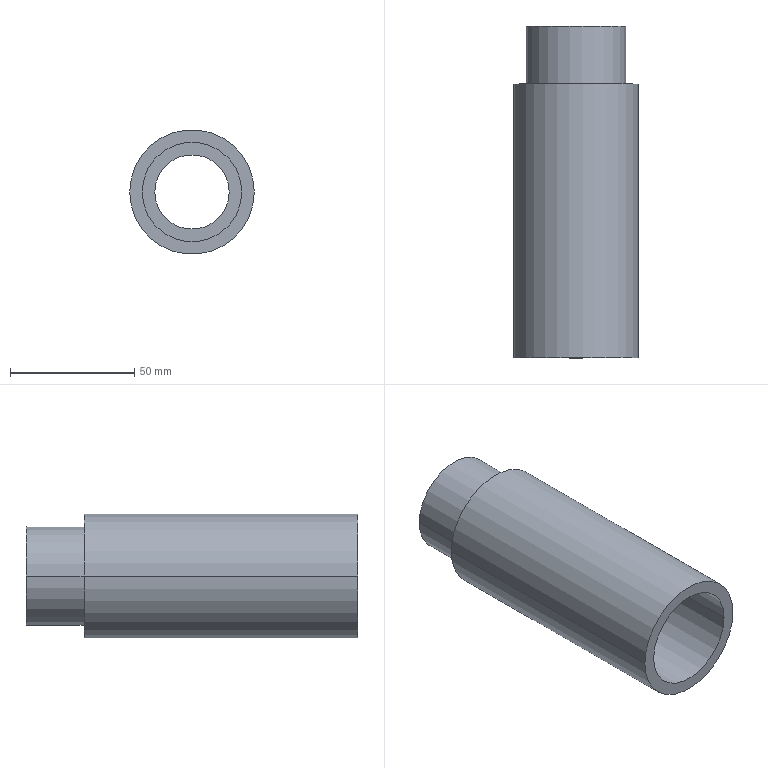Part | SolidWorks | features Revolution 1 | 1 solid | 12 faces | box 50 x 133.28 x 50 mm | volume 92984 mm3 | cylinder 8 | plane 4 | commonest cylinder face diameters 29.9 x2 39.9 x2 40 x2 50 x2
STEP:
#1=CARTESIAN_POINT('',(91.067,-25.489,0.));
#2=VERTEX_POINT('',#1);
#3=CARTESIAN_POINT('',(51.067,-25.489,0.));
#4=VERTEX_POINT('',#3);
#5=CARTESIAN_POINT('',(71.067,-25.489,0.));
#6=DIRECTION('',(0.,1.,0.));
#7=DIRECTION('',(-1.,0.,0.));
#8=AXIS2_PLACEMENT_3D('',#5,#6,#7);
#9=CIRCLE('',#8,20.);
#10=EDGE_CURVE('',#2,#4,#9,.T.);
#11=ORIENTED_EDGE('',*,*,#10,.F.);
#12=CARTESIAN_POINT('',(91.067,80.061,0.));
#13=VERTEX_POINT('',#12);
#14=CARTESIAN_POINT('',(91.067,101.178,0.));
#15=DIRECTION('',(0.,1.,0.));
#16=VECTOR('',#15,1000.);
#17=LINE('',#14,#16);
#18=EDGE_CURVE('',#2,#13,#17,.T.);
#19=ORIENTED_EDGE('',*,*,#18,.T.);
#20=CARTESIAN_POINT('',(51.067,80.061,0.));
#21=VERTEX_POINT('',#20);
#22=CARTESIAN_POINT('',(71.067,80.061,0.));
#23=DIRECTION('',(0.,1.,0.));
#24=DIRECTION('',(-1.,0.,0.));
#25=AXIS2_PLACEMENT_3D('',#22,#23,#24);
#26=CIRCLE('',#25,20.);
#27=EDGE_CURVE('',#13,#21,#26,.T.);
#28=ORIENTED_EDGE('',*,*,#27,.T.);
#29=CARTESIAN_POINT('',(51.067,101.178,0.));
#30=DIRECTION('',(0.,1.,0.));
#31=VECTOR('',#30,1000.);
#32=LINE('',#29,#31);
#33=EDGE_CURVE('',#4,#21,#32,.T.);
#34=ORIENTED_EDGE('',*,*,#33,.F.);
#35=EDGE_LOOP('',(#11,#19,#28,#34));
#36=FACE_OUTER_BOUND('',#35,.T.);
#37=CARTESIAN_POINT('',(71.067,101.178,0.));
#38=DIRECTION('',(0.,1.,0.));
#39=DIRECTION('',(-1.,0.,0.));
#40=AXIS2_PLACEMENT_3D('',#37,#38,#39);
#41=CYLINDRICAL_SURFACE('',#40,20.);
#42=ADVANCED_FACE('',(#36),#41,.F.);
#43=CARTESIAN_POINT('',(86.017,80.061,0.));
#44=VERTEX_POINT('',#43);
#45=CARTESIAN_POINT('',(56.117,80.061,0.));
#46=VERTEX_POINT('',#45);
#47=CARTESIAN_POINT('',(71.067,80.061,0.));
#48=DIRECTION('',(0.,1.,0.));
#49=DIRECTION('',(-1.,0.,0.));
#50=AXIS2_PLACEMENT_3D('',#47,#48,#49);
#51=CIRCLE('',#50,14.95);
#52=EDGE_CURVE('',#44,#46,#51,.T.);
#53=ORIENTED_EDGE('',*,*,#52,.F.);
#54=CARTESIAN_POINT('',(86.017,107.791,0.));
#55=VERTEX_POINT('',#54);
#56=CARTESIAN_POINT('',(86.017,101.178,0.));
#57=DIRECTION('',(0.,1.,0.));
#58=VECTOR('',#57,1000.);
#59=LINE('',#56,#58);
#60=EDGE_CURVE('',#44,#55,#59,.T.);
#61=ORIENTED_EDGE('',*,*,#60,.T.);
#62=CARTESIAN_POINT('',(56.117,107.791,0.));
#63=VERTEX_POINT('',#62);
#64=CARTESIAN_POINT('',(71.067,107.791,0.));
#65=DIRECTION('',(0.,1.,0.));
#66=DIRECTION('',(-1.,0.,0.));
#67=AXIS2_PLACEMENT_3D('',#64,#65,#66);
#68=CIRCLE('',#67,14.95);
#69=EDGE_CURVE('',#55,#63,#68,.T.);
#70=ORIENTED_EDGE('',*,*,#69,.T.);
#71=CARTESIAN_POINT('',(56.117,101.178,0.));
#72=DIRECTION('',(0.,1.,0.));
#73=VECTOR('',#72,1000.);
#74=LINE('',#71,#73);
#75=EDGE_CURVE('',#46,#63,#74,.T.);
#76=ORIENTED_EDGE('',*,*,#75,.F.);
#77=EDGE_LOOP('',(#53,#61,#70,#76));
#78=FACE_OUTER_BOUND('',#77,.T.);
#79=CARTESIAN_POINT('',(71.067,101.178,0.));
#80=DIRECTION('',(0.,1.,0.));
#81=DIRECTION('',(-1.,0.,0.));
#82=AXIS2_PLACEMENT_3D('',#79,#80,#81);
#83=CYLINDRICAL_SURFACE('',#82,14.95);
#84=ADVANCED_FACE('',(#78),#83,.F.);
#85=CARTESIAN_POINT('',(51.117,84.511,0.));
#86=VERTEX_POINT('',#85);
#87=CARTESIAN_POINT('',(91.017,84.511,0.));
#88=VERTEX_POINT('',#87);
#89=CARTESIAN_POINT('',(71.067,84.511,0.));
#90=DIRECTION('',(0.,1.,0.));
#91=DIRECTION('',(-1.,0.,0.));
#92=AXIS2_PLACEMENT_3D('',#89,#90,#91);
#93=CIRCLE('',#92,19.95);
#94=EDGE_CURVE('',#86,#88,#93,.T.);
#95=ORIENTED_EDGE('',*,*,#94,.T.);
#96=CARTESIAN_POINT('',(91.017,107.791,0.));
#97=VERTEX_POINT('',#96);
#98=CARTESIAN_POINT('',(91.017,101.178,0.));
#99=DIRECTION('',(0.,1.,0.));
#100=VECTOR('',#99,1000.);
#101=LINE('',#98,#100);
#102=EDGE_CURVE('',#88,#97,#101,.T.);
#103=ORIENTED_EDGE('',*,*,#102,.T.);
#104=CARTESIAN_POINT('',(51.117,107.791,0.));
#105=VERTEX_POINT('',#104);
#106=CARTESIAN_POINT('',(71.067,107.791,0.));
#107=DIRECTION('',(0.,1.,0.));
#108=DIRECTION('',(-1.,0.,0.));
#109=AXIS2_PLACEMENT_3D('',#106,#107,#108);
#110=CIRCLE('',#109,19.95);
#111=EDGE_CURVE('',#105,#97,#110,.T.);
#112=ORIENTED_EDGE('',*,*,#111,.F.);
#113=CARTESIAN_POINT('',(51.117,101.178,0.));
#114=DIRECTION('',(0.,1.,0.));
#115=VECTOR('',#114,1000.);
#116=LINE('',#113,#115);
#117=EDGE_CURVE('',#86,#105,#116,.T.);
#118=ORIENTED_EDGE('',*,*,#117,.F.);
#119=EDGE_LOOP('',(#95,#103,#112,#118));
#120=FACE_OUTER_BOUND('',#119,.T.);
#121=CARTESIAN_POINT('',(71.067,101.178,0.));
#122=DIRECTION('',(0.,1.,0.));
#123=DIRECTION('',(-1.,0.,0.));
#124=AXIS2_PLACEMENT_3D('',#121,#122,#123);
#125=CYLINDRICAL_SURFACE('',#124,19.95);
#126=ADVANCED_FACE('',(#120),#125,.T.);
#127=CARTESIAN_POINT('',(46.067,-25.489,0.));
#128=VERTEX_POINT('',#127);
#129=CARTESIAN_POINT('',(96.067,-25.489,0.));
#130=VERTEX_POINT('',#129);
#131=CARTESIAN_POINT('',(71.067,-25.489,0.));
#132=DIRECTION('',(0.,1.,0.));
#133=DIRECTION('',(-1.,0.,0.));
#134=AXIS2_PLACEMENT_3D('',#131,#132,#133);
#135=CIRCLE('',#134,25.);
#136=EDGE_CURVE('',#128,#130,#135,.T.);
#137=ORIENTED_EDGE('',*,*,#136,.T.);
#138=CARTESIAN_POINT('',(96.067,84.511,0.));
#139=VERTEX_POINT('',#138);
#140=CARTESIAN_POINT('',(96.067,101.178,0.));
#141=DIRECTION('',(0.,1.,0.));
#142=VECTOR('',#141,1000.);
#143=LINE('',#140,#142);
#144=EDGE_CURVE('',#130,#139,#143,.T.);
#145=ORIENTED_EDGE('',*,*,#144,.T.);
#146=CARTESIAN_POINT('',(46.067,84.511,0.));
#147=VERTEX_POINT('',#146);
#148=CARTESIAN_POINT('',(71.067,84.511,0.));
#149=DIRECTION('',(0.,1.,0.));
#150=DIRECTION('',(-1.,0.,0.));
#151=AXIS2_PLACEMENT_3D('',#148,#149,#150);
#152=CIRCLE('',#151,25.);
#153=EDGE_CURVE('',#147,#139,#152,.T.);
#154=ORIENTED_EDGE('',*,*,#153,.F.);
#155=CARTESIAN_POINT('',(46.067,101.178,0.));
#156=DIRECTION('',(0.,1.,0.));
#157=VECTOR('',#156,1000.);
#158=LINE('',#155,#157);
#159=EDGE_CURVE('',#128,#147,#158,.T.);
#160=ORIENTED_EDGE('',*,*,#159,.F.);
#161=EDGE_LOOP('',(#137,#145,#154,#160));
#162=FACE_OUTER_BOUND('',#161,.T.);
#163=CARTESIAN_POINT('',(71.067,101.178,0.));
#164=DIRECTION('',(0.,1.,0.));
#165=DIRECTION('',(-1.,0.,0.));
#166=AXIS2_PLACEMENT_3D('',#163,#164,#165);
#167=CYLINDRICAL_SURFACE('',#166,25.);
#168=ADVANCED_FACE('',(#162),#167,.T.);
#169=CARTESIAN_POINT('',(71.067,-25.489,0.));
#170=DIRECTION('',(0.,1.,0.));
#171=DIRECTION('',(-1.,0.,0.));
#172=AXIS2_PLACEMENT_3D('',#169,#170,#171);
#173=CIRCLE('',#172,20.);
#174=EDGE_CURVE('',#4,#2,#173,.T.);
#175=ORIENTED_EDGE('',*,*,#174,.T.);
#176=ORIENTED_EDGE('',*,*,#10,.T.);
#177=EDGE_LOOP('',(#175,#176));
#178=FACE_BOUND('',#177,.T.);
#179=ORIENTED_EDGE('',*,*,#136,.F.);
#180=CARTESIAN_POINT('',(71.067,-25.489,0.));
#181=DIRECTION('',(0.,1.,0.));
#182=DIRECTION('',(-1.,0.,0.));
#183=AXIS2_PLACEMENT_3D('',#180,#181,#182);
#184=CIRCLE('',#183,25.);
#185=EDGE_CURVE('',#130,#128,#184,.T.);
#186=ORIENTED_EDGE('',*,*,#185,.F.);
#187=EDGE_LOOP('',(#179,#186));
#188=FACE_OUTER_BOUND('',#187,.T.);
#189=CARTESIAN_POINT('',(51.067,-25.489,0.));
#190=DIRECTION('',(0.,-1.,0.));
#191=DIRECTION('',(1.,0.,0.));
#192=AXIS2_PLACEMENT_3D('',#189,#190,#191);
#193=PLANE('',#192);
#194=ADVANCED_FACE('',(#178,#188),#193,.T.);
#195=ORIENTED_EDGE('',*,*,#144,.F.);
#196=ORIENTED_EDGE('',*,*,#185,.T.);
#197=ORIENTED_EDGE('',*,*,#159,.T.);
#198=CARTESIAN_POINT('',(71.067,84.511,0.));
#199=DIRECTION('',(0.,1.,0.));
#200=DIRECTION('',(-1.,0.,0.));
#201=AXIS2_PLACEMENT_3D('',#198,#199,#200);
#202=CIRCLE('',#201,25.);
#203=EDGE_CURVE('',#139,#147,#202,.T.);
#204=ORIENTED_EDGE('',*,*,#203,.F.);
#205=EDGE_LOOP('',(#195,#196,#197,#204));
#206=FACE_OUTER_BOUND('',#205,.T.);
#207=CARTESIAN_POINT('',(71.067,101.178,0.));
#208=DIRECTION('',(0.,1.,0.));
#209=DIRECTION('',(-1.,0.,0.));
#210=AXIS2_PLACEMENT_3D('',#207,#208,#209);
#211=CYLINDRICAL_SURFACE('',#210,25.);
#212=ADVANCED_FACE('',(#206),#211,.T.);
#213=ORIENTED_EDGE('',*,*,#153,.T.);
#214=ORIENTED_EDGE('',*,*,#203,.T.);
#215=EDGE_LOOP('',(#213,#214));
#216=FACE_OUTER_BOUND('',#215,.T.);
#217=ORIENTED_EDGE('',*,*,#94,.F.);
#218=CARTESIAN_POINT('',(71.067,84.511,0.));
#219=DIRECTION('',(0.,1.,0.));
#220=DIRECTION('',(-1.,0.,0.));
#221=AXIS2_PLACEMENT_3D('',#218,#219,#220);
#222=CIRCLE('',#221,19.95);
#223=EDGE_CURVE('',#88,#86,#222,.T.);
#224=ORIENTED_EDGE('',*,*,#223,.F.);
#225=EDGE_LOOP('',(#217,#224));
#226=FACE_BOUND('',#225,.T.);
#227=CARTESIAN_POINT('',(51.117,84.511,0.));
#228=DIRECTION('',(0.,1.,0.));
#229=DIRECTION('',(-1.,0.,0.));
#230=AXIS2_PLACEMENT_3D('',#227,#228,#229);
#231=PLANE('',#230);
#232=ADVANCED_FACE('',(#216,#226),#231,.T.);
#233=ORIENTED_EDGE('',*,*,#102,.F.);
#234=ORIENTED_EDGE('',*,*,#223,.T.);
#235=ORIENTED_EDGE('',*,*,#117,.T.);
#236=CARTESIAN_POINT('',(71.067,107.791,0.));
#237=DIRECTION('',(0.,1.,0.));
#238=DIRECTION('',(-1.,0.,0.));
#239=AXIS2_PLACEMENT_3D('',#236,#237,#238);
#240=CIRCLE('',#239,19.95);
#241=EDGE_CURVE('',#97,#105,#240,.T.);
#242=ORIENTED_EDGE('',*,*,#241,.F.);
#243=EDGE_LOOP('',(#233,#234,#235,#242));
#244=FACE_OUTER_BOUND('',#243,.T.);
#245=CARTESIAN_POINT('',(71.067,101.178,0.));
#246=DIRECTION('',(0.,1.,0.));
#247=DIRECTION('',(-1.,0.,0.));
#248=AXIS2_PLACEMENT_3D('',#245,#246,#247);
#249=CYLINDRICAL_SURFACE('',#248,19.95);
#250=ADVANCED_FACE('',(#244),#249,.T.);
#251=ORIENTED_EDGE('',*,*,#111,.T.);
#252=ORIENTED_EDGE('',*,*,#241,.T.);
#253=EDGE_LOOP('',(#251,#252));
#254=FACE_OUTER_BOUND('',#253,.T.);
#255=CARTESIAN_POINT('',(71.067,107.791,0.));
#256=DIRECTION('',(0.,1.,0.));
#257=DIRECTION('',(-1.,0.,0.));
#258=AXIS2_PLACEMENT_3D('',#255,#256,#257);
#259=CIRCLE('',#258,14.95);
#260=EDGE_CURVE('',#63,#55,#259,.T.);
#261=ORIENTED_EDGE('',*,*,#260,.F.);
#262=ORIENTED_EDGE('',*,*,#69,.F.);
#263=EDGE_LOOP('',(#261,#262));
#264=FACE_BOUND('',#263,.T.);
#265=CARTESIAN_POINT('',(51.117,107.791,0.));
#266=DIRECTION('',(0.,1.,0.));
#267=DIRECTION('',(-1.,0.,0.));
#268=AXIS2_PLACEMENT_3D('',#265,#266,#267);
#269=PLANE('',#268);
#270=ADVANCED_FACE('',(#254,#264),#269,.T.);
#271=ORIENTED_EDGE('',*,*,#60,.F.);
#272=CARTESIAN_POINT('',(71.067,80.061,0.));
#273=DIRECTION('',(0.,1.,0.));
#274=DIRECTION('',(-1.,0.,0.));
#275=AXIS2_PLACEMENT_3D('',#272,#273,#274);
#276=CIRCLE('',#275,14.95);
#277=EDGE_CURVE('',#46,#44,#276,.T.);
#278=ORIENTED_EDGE('',*,*,#277,.F.);
#279=ORIENTED_EDGE('',*,*,#75,.T.);
#280=ORIENTED_EDGE('',*,*,#260,.T.);
#281=EDGE_LOOP('',(#271,#278,#279,#280));
#282=FACE_OUTER_BOUND('',#281,.T.);
#283=CARTESIAN_POINT('',(71.067,101.178,0.));
#284=DIRECTION('',(0.,1.,0.));
#285=DIRECTION('',(-1.,0.,0.));
#286=AXIS2_PLACEMENT_3D('',#283,#284,#285);
#287=CYLINDRICAL_SURFACE('',#286,14.95);
#288=ADVANCED_FACE('',(#282),#287,.F.);
#289=ORIENTED_EDGE('',*,*,#277,.T.);
#290=ORIENTED_EDGE('',*,*,#52,.T.);
#291=EDGE_LOOP('',(#289,#290));
#292=FACE_BOUND('',#291,.T.);
#293=CARTESIAN_POINT('',(71.067,80.061,0.));
#294=DIRECTION('',(0.,1.,0.));
#295=DIRECTION('',(-1.,0.,0.));
#296=AXIS2_PLACEMENT_3D('',#293,#294,#295);
#297=CIRCLE('',#296,20.);
#298=EDGE_CURVE('',#21,#13,#297,.T.);
#299=ORIENTED_EDGE('',*,*,#298,.F.);
#300=ORIENTED_EDGE('',*,*,#27,.F.);
#301=EDGE_LOOP('',(#299,#300));
#302=FACE_OUTER_BOUND('',#301,.T.);
#303=CARTESIAN_POINT('',(51.067,80.061,0.));
#304=DIRECTION('',(0.,-1.,0.));
#305=DIRECTION('',(1.,0.,0.));
#306=AXIS2_PLACEMENT_3D('',#303,#304,#305);
#307=PLANE('',#306);
#308=ADVANCED_FACE('',(#292,#302),#307,.T.);
#309=ORIENTED_EDGE('',*,*,#18,.F.);
#310=ORIENTED_EDGE('',*,*,#174,.F.);
#311=ORIENTED_EDGE('',*,*,#33,.T.);
#312=ORIENTED_EDGE('',*,*,#298,.T.);
#313=EDGE_LOOP('',(#309,#310,#311,#312));
#314=FACE_OUTER_BOUND('',#313,.T.);
#315=CARTESIAN_POINT('',(71.067,101.178,0.));
#316=DIRECTION('',(0.,1.,0.));
#317=DIRECTION('',(-1.,0.,0.));
#318=AXIS2_PLACEMENT_3D('',#315,#316,#317);
#319=CYLINDRICAL_SURFACE('',#318,20.);
#320=ADVANCED_FACE('',(#314),#319,.F.);
#321=CLOSED_SHELL('',(#42,#84,#126,#168,#194,#212,#232,#250,#270,#288,#308,#320));
#322=MANIFOLD_SOLID_BREP('',#321);
#323=CARTESIAN_POINT('',(0.,0.,0.));
#324=DIRECTION('',(0.,0.,1.));
#325=DIRECTION('',(1.,0.,0.));
#326=AXIS2_PLACEMENT_3D('',#323,#324,#325);
#327=(LENGTH_UNIT()NAMED_UNIT(*)SI_UNIT(.MILLI.,.METRE.));
#328=UNCERTAINTY_MEASURE_WITH_UNIT(LENGTH_MEASURE(0.00001),#327,'','');
#329=(NAMED_UNIT(*)PLANE_ANGLE_UNIT()SI_UNIT($,.RADIAN.));
#330=(NAMED_UNIT(*)SI_UNIT($,.STERADIAN.)SOLID_ANGLE_UNIT());
#331=(GEOMETRIC_REPRESENTATION_CONTEXT(3)GLOBAL_UNCERTAINTY_ASSIGNED_CONTEXT((#328))GLOBAL_UNIT_ASSIGNED_CONTEXT((#327,#329,#330))REPRESENTATION_CONTEXT('',''));
#332=ADVANCED_BREP_SHAPE_REPRESENTATION('',(#322,#326),#331);